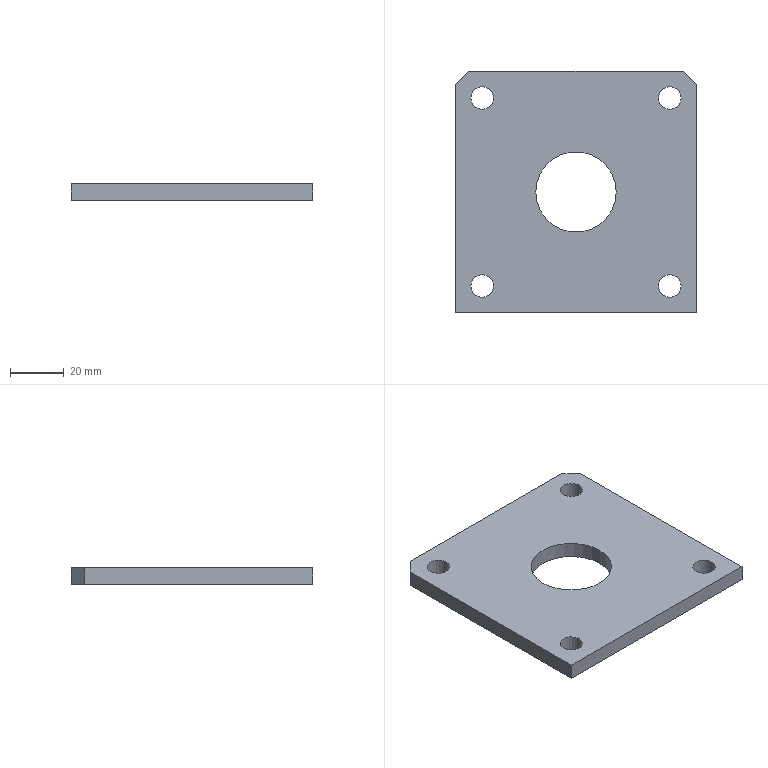Part | STEP file | backplate | 1 solid | 13 faces | box 90 x 90 x 6 mm | volume 42888 mm3 | plane 8 | spline 5